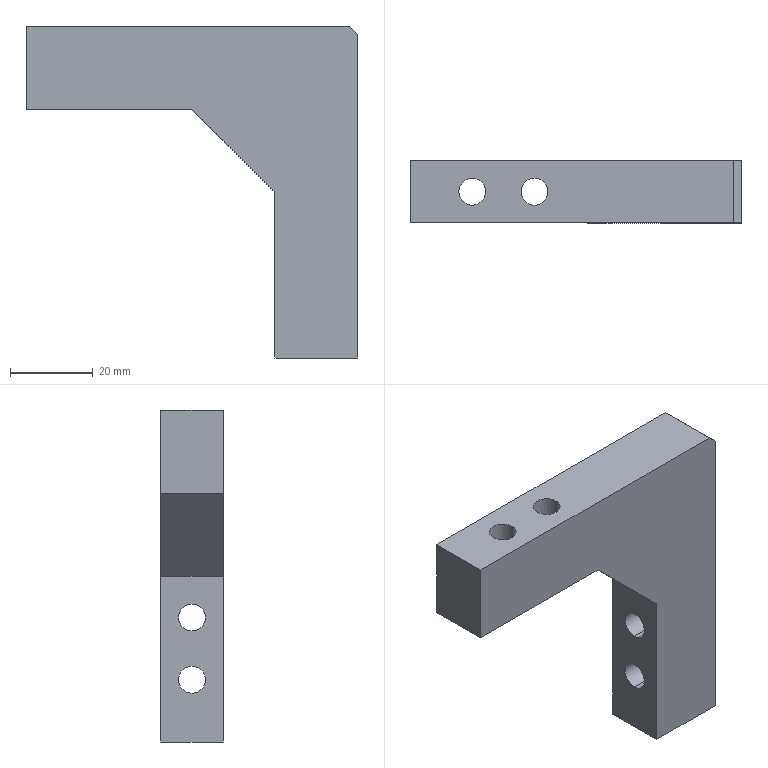Part | SolidWorks | features ICE 2, LPattern 2, Chamfer 1, Extrusion 1 | 1 solid | 18 faces | box 80 x 15 x 80 mm | volume 42315 mm3 | plane 10 | cylinder 8 | commonest cylinder face diameters 6.5 x8
STEP:
#1=CARTESIAN_POINT('',(20.,7.5,-21.75));
#2=VERTEX_POINT('',#1);
#3=CARTESIAN_POINT('',(20.,7.5,-28.25));
#4=VERTEX_POINT('',#3);
#5=CARTESIAN_POINT('',(20.,7.5,-25.));
#6=DIRECTION('',(1.,0.,0.));
#7=DIRECTION('',(0.,0.,-1.));
#8=AXIS2_PLACEMENT_3D('',#5,#6,#7);
#9=CIRCLE('',#8,3.25);
#10=EDGE_CURVE('',#2,#4,#9,.T.);
#11=ORIENTED_EDGE('',*,*,#10,.F.);
#12=CARTESIAN_POINT('',(40.,7.5,-21.75));
#13=VERTEX_POINT('',#12);
#14=CARTESIAN_POINT('',(-40.,7.5,-21.75));
#15=DIRECTION('',(1.,0.,0.));
#16=VECTOR('',#15,1000.);
#17=LINE('',#14,#16);
#18=EDGE_CURVE('',#2,#13,#17,.T.);
#19=ORIENTED_EDGE('',*,*,#18,.T.);
#20=CARTESIAN_POINT('',(40.,7.5,-28.25));
#21=VERTEX_POINT('',#20);
#22=CARTESIAN_POINT('',(40.,7.5,-25.));
#23=DIRECTION('',(1.,0.,0.));
#24=DIRECTION('',(0.,0.,-1.));
#25=AXIS2_PLACEMENT_3D('',#22,#23,#24);
#26=CIRCLE('',#25,3.25);
#27=EDGE_CURVE('',#13,#21,#26,.T.);
#28=ORIENTED_EDGE('',*,*,#27,.T.);
#29=CARTESIAN_POINT('',(-40.,7.5,-28.25));
#30=DIRECTION('',(1.,0.,0.));
#31=VECTOR('',#30,1000.);
#32=LINE('',#29,#31);
#33=EDGE_CURVE('',#4,#21,#32,.T.);
#34=ORIENTED_EDGE('',*,*,#33,.F.);
#35=EDGE_LOOP('',(#11,#19,#28,#34));
#36=FACE_OUTER_BOUND('',#35,.T.);
#37=CARTESIAN_POINT('',(-40.,7.5,-25.));
#38=DIRECTION('',(1.,0.,0.));
#39=DIRECTION('',(0.,0.,-1.));
#40=AXIS2_PLACEMENT_3D('',#37,#38,#39);
#41=CYLINDRICAL_SURFACE('',#40,3.25);
#42=ADVANCED_FACE('',(#36),#41,.F.);
#43=CARTESIAN_POINT('',(20.,7.5,-6.75));
#44=VERTEX_POINT('',#43);
#45=CARTESIAN_POINT('',(20.,7.5,-13.25));
#46=VERTEX_POINT('',#45);
#47=CARTESIAN_POINT('',(20.,7.5,-10.));
#48=DIRECTION('',(1.,0.,0.));
#49=DIRECTION('',(0.,0.,-1.));
#50=AXIS2_PLACEMENT_3D('',#47,#48,#49);
#51=CIRCLE('',#50,3.25);
#52=EDGE_CURVE('',#44,#46,#51,.T.);
#53=ORIENTED_EDGE('',*,*,#52,.F.);
#54=CARTESIAN_POINT('',(40.,7.5,-6.75));
#55=VERTEX_POINT('',#54);
#56=CARTESIAN_POINT('',(-40.,7.5,-6.75));
#57=DIRECTION('',(1.,0.,0.));
#58=VECTOR('',#57,1000.);
#59=LINE('',#56,#58);
#60=EDGE_CURVE('',#44,#55,#59,.T.);
#61=ORIENTED_EDGE('',*,*,#60,.T.);
#62=CARTESIAN_POINT('',(40.,7.5,-13.25));
#63=VERTEX_POINT('',#62);
#64=CARTESIAN_POINT('',(40.,7.5,-10.));
#65=DIRECTION('',(1.,0.,0.));
#66=DIRECTION('',(0.,0.,-1.));
#67=AXIS2_PLACEMENT_3D('',#64,#65,#66);
#68=CIRCLE('',#67,3.25);
#69=EDGE_CURVE('',#55,#63,#68,.T.);
#70=ORIENTED_EDGE('',*,*,#69,.T.);
#71=CARTESIAN_POINT('',(-40.,7.5,-13.25));
#72=DIRECTION('',(1.,0.,0.));
#73=VECTOR('',#72,1000.);
#74=LINE('',#71,#73);
#75=EDGE_CURVE('',#46,#63,#74,.T.);
#76=ORIENTED_EDGE('',*,*,#75,.F.);
#77=EDGE_LOOP('',(#53,#61,#70,#76));
#78=FACE_OUTER_BOUND('',#77,.T.);
#79=CARTESIAN_POINT('',(-40.,7.5,-10.));
#80=DIRECTION('',(1.,0.,0.));
#81=DIRECTION('',(0.,0.,-1.));
#82=AXIS2_PLACEMENT_3D('',#79,#80,#81);
#83=CYLINDRICAL_SURFACE('',#82,3.25);
#84=ADVANCED_FACE('',(#78),#83,.F.);
#85=CARTESIAN_POINT('',(-21.75,7.5,40.));
#86=VERTEX_POINT('',#85);
#87=CARTESIAN_POINT('',(-28.25,7.5,40.));
#88=VERTEX_POINT('',#87);
#89=CARTESIAN_POINT('',(-25.,7.5,40.));
#90=DIRECTION('',(0.,0.,-1.));
#91=DIRECTION('',(-1.,0.,0.));
#92=AXIS2_PLACEMENT_3D('',#89,#90,#91);
#93=CIRCLE('',#92,3.25);
#94=EDGE_CURVE('',#86,#88,#93,.T.);
#95=ORIENTED_EDGE('',*,*,#94,.F.);
#96=CARTESIAN_POINT('',(-21.75,7.5,20.));
#97=VERTEX_POINT('',#96);
#98=CARTESIAN_POINT('',(-21.75,7.5,40.));
#99=DIRECTION('',(0.,0.,-1.));
#100=VECTOR('',#99,1000.);
#101=LINE('',#98,#100);
#102=EDGE_CURVE('',#86,#97,#101,.T.);
#103=ORIENTED_EDGE('',*,*,#102,.T.);
#104=CARTESIAN_POINT('',(-28.25,7.5,20.));
#105=VERTEX_POINT('',#104);
#106=CARTESIAN_POINT('',(-25.,7.5,20.));
#107=DIRECTION('',(0.,0.,-1.));
#108=DIRECTION('',(-1.,0.,0.));
#109=AXIS2_PLACEMENT_3D('',#106,#107,#108);
#110=CIRCLE('',#109,3.25);
#111=EDGE_CURVE('',#97,#105,#110,.T.);
#112=ORIENTED_EDGE('',*,*,#111,.T.);
#113=CARTESIAN_POINT('',(-28.25,7.5,40.));
#114=DIRECTION('',(0.,0.,-1.));
#115=VECTOR('',#114,1000.);
#116=LINE('',#113,#115);
#117=EDGE_CURVE('',#88,#105,#116,.T.);
#118=ORIENTED_EDGE('',*,*,#117,.F.);
#119=EDGE_LOOP('',(#95,#103,#112,#118));
#120=FACE_OUTER_BOUND('',#119,.T.);
#121=CARTESIAN_POINT('',(-25.,7.5,40.));
#122=DIRECTION('',(0.,0.,-1.));
#123=DIRECTION('',(-1.,0.,0.));
#124=AXIS2_PLACEMENT_3D('',#121,#122,#123);
#125=CYLINDRICAL_SURFACE('',#124,3.25);
#126=ADVANCED_FACE('',(#120),#125,.F.);
#127=CARTESIAN_POINT('',(-6.75,7.5,40.));
#128=VERTEX_POINT('',#127);
#129=CARTESIAN_POINT('',(-13.25,7.5,40.));
#130=VERTEX_POINT('',#129);
#131=CARTESIAN_POINT('',(-10.,7.5,40.));
#132=DIRECTION('',(0.,0.,-1.));
#133=DIRECTION('',(-1.,0.,0.));
#134=AXIS2_PLACEMENT_3D('',#131,#132,#133);
#135=CIRCLE('',#134,3.25);
#136=EDGE_CURVE('',#128,#130,#135,.T.);
#137=ORIENTED_EDGE('',*,*,#136,.F.);
#138=CARTESIAN_POINT('',(-6.75,7.5,20.));
#139=VERTEX_POINT('',#138);
#140=CARTESIAN_POINT('',(-6.75,7.5,40.));
#141=DIRECTION('',(0.,0.,-1.));
#142=VECTOR('',#141,1000.);
#143=LINE('',#140,#142);
#144=EDGE_CURVE('',#128,#139,#143,.T.);
#145=ORIENTED_EDGE('',*,*,#144,.T.);
#146=CARTESIAN_POINT('',(-13.25,7.5,20.));
#147=VERTEX_POINT('',#146);
#148=CARTESIAN_POINT('',(-10.,7.5,20.));
#149=DIRECTION('',(0.,0.,-1.));
#150=DIRECTION('',(-1.,0.,0.));
#151=AXIS2_PLACEMENT_3D('',#148,#149,#150);
#152=CIRCLE('',#151,3.25);
#153=EDGE_CURVE('',#139,#147,#152,.T.);
#154=ORIENTED_EDGE('',*,*,#153,.T.);
#155=CARTESIAN_POINT('',(-13.25,7.5,40.));
#156=DIRECTION('',(0.,0.,-1.));
#157=VECTOR('',#156,1000.);
#158=LINE('',#155,#157);
#159=EDGE_CURVE('',#130,#147,#158,.T.);
#160=ORIENTED_EDGE('',*,*,#159,.F.);
#161=EDGE_LOOP('',(#137,#145,#154,#160));
#162=FACE_OUTER_BOUND('',#161,.T.);
#163=CARTESIAN_POINT('',(-10.,7.5,40.));
#164=DIRECTION('',(0.,0.,-1.));
#165=DIRECTION('',(-1.,0.,0.));
#166=AXIS2_PLACEMENT_3D('',#163,#164,#165);
#167=CYLINDRICAL_SURFACE('',#166,3.25);
#168=ADVANCED_FACE('',(#162),#167,.F.);
#169=CARTESIAN_POINT('',(40.,7.5,-25.));
#170=DIRECTION('',(1.,0.,0.));
#171=DIRECTION('',(0.,0.,-1.));
#172=AXIS2_PLACEMENT_3D('',#169,#170,#171);
#173=CIRCLE('',#172,3.25);
#174=EDGE_CURVE('',#21,#13,#173,.T.);
#175=ORIENTED_EDGE('',*,*,#174,.F.);
#176=ORIENTED_EDGE('',*,*,#27,.F.);
#177=EDGE_LOOP('',(#175,#176));
#178=FACE_BOUND('',#177,.T.);
#179=CARTESIAN_POINT('',(40.,7.5,-10.));
#180=DIRECTION('',(1.,0.,0.));
#181=DIRECTION('',(0.,0.,-1.));
#182=AXIS2_PLACEMENT_3D('',#179,#180,#181);
#183=CIRCLE('',#182,3.25);
#184=EDGE_CURVE('',#63,#55,#183,.T.);
#185=ORIENTED_EDGE('',*,*,#184,.F.);
#186=ORIENTED_EDGE('',*,*,#69,.F.);
#187=EDGE_LOOP('',(#185,#186));
#188=FACE_BOUND('',#187,.T.);
#189=CARTESIAN_POINT('',(40.,15.,38.));
#190=VERTEX_POINT('',#189);
#191=CARTESIAN_POINT('',(40.,15.,-40.));
#192=VERTEX_POINT('',#191);
#193=CARTESIAN_POINT('',(40.,15.,40.));
#194=DIRECTION('',(0.,0.,-1.));
#195=VECTOR('',#194,1000.);
#196=LINE('',#193,#195);
#197=EDGE_CURVE('',#190,#192,#196,.T.);
#198=ORIENTED_EDGE('',*,*,#197,.F.);
#199=CARTESIAN_POINT('',(40.,0.,38.));
#200=VERTEX_POINT('',#199);
#201=CARTESIAN_POINT('',(40.,15.,38.));
#202=DIRECTION('',(0.,-1.,0.));
#203=VECTOR('',#202,1000.);
#204=LINE('',#201,#203);
#205=EDGE_CURVE('',#190,#200,#204,.T.);
#206=ORIENTED_EDGE('',*,*,#205,.T.);
#207=CARTESIAN_POINT('',(40.,0.,-40.));
#208=VERTEX_POINT('',#207);
#209=CARTESIAN_POINT('',(40.,0.,40.));
#210=DIRECTION('',(0.,0.,-1.));
#211=VECTOR('',#210,1000.);
#212=LINE('',#209,#211);
#213=EDGE_CURVE('',#200,#208,#212,.T.);
#214=ORIENTED_EDGE('',*,*,#213,.T.);
#215=CARTESIAN_POINT('',(40.,15.,-40.));
#216=DIRECTION('',(0.,-1.,0.));
#217=VECTOR('',#216,1000.);
#218=LINE('',#215,#217);
#219=EDGE_CURVE('',#192,#208,#218,.T.);
#220=ORIENTED_EDGE('',*,*,#219,.F.);
#221=EDGE_LOOP('',(#198,#206,#214,#220));
#222=FACE_OUTER_BOUND('',#221,.T.);
#223=CARTESIAN_POINT('',(40.,15.,40.));
#224=DIRECTION('',(-1.,0.,0.));
#225=DIRECTION('',(0.,0.,1.));
#226=AXIS2_PLACEMENT_3D('',#223,#224,#225);
#227=PLANE('',#226);
#228=ADVANCED_FACE('',(#178,#188,#222),#227,.F.);
#229=CARTESIAN_POINT('',(20.,0.,-40.));
#230=VERTEX_POINT('',#229);
#231=CARTESIAN_POINT('',(40.,0.,-40.));
#232=DIRECTION('',(-1.,0.,0.));
#233=VECTOR('',#232,1000.);
#234=LINE('',#231,#233);
#235=EDGE_CURVE('',#208,#230,#234,.T.);
#236=ORIENTED_EDGE('',*,*,#235,.T.);
#237=CARTESIAN_POINT('',(20.,15.,-40.));
#238=VERTEX_POINT('',#237);
#239=CARTESIAN_POINT('',(20.,15.,-40.));
#240=DIRECTION('',(0.,-1.,0.));
#241=VECTOR('',#240,1000.);
#242=LINE('',#239,#241);
#243=EDGE_CURVE('',#238,#230,#242,.T.);
#244=ORIENTED_EDGE('',*,*,#243,.F.);
#245=CARTESIAN_POINT('',(40.,15.,-40.));
#246=DIRECTION('',(-1.,0.,0.));
#247=VECTOR('',#246,1000.);
#248=LINE('',#245,#247);
#249=EDGE_CURVE('',#192,#238,#248,.T.);
#250=ORIENTED_EDGE('',*,*,#249,.F.);
#251=ORIENTED_EDGE('',*,*,#219,.T.);
#252=EDGE_LOOP('',(#236,#244,#250,#251));
#253=FACE_OUTER_BOUND('',#252,.T.);
#254=CARTESIAN_POINT('',(40.,15.,-40.));
#255=DIRECTION('',(0.,0.,1.));
#256=DIRECTION('',(1.,0.,0.));
#257=AXIS2_PLACEMENT_3D('',#254,#255,#256);
#258=PLANE('',#257);
#259=ADVANCED_FACE('',(#253),#258,.F.);
#260=CARTESIAN_POINT('',(20.,7.5,-25.));
#261=DIRECTION('',(1.,0.,0.));
#262=DIRECTION('',(0.,0.,-1.));
#263=AXIS2_PLACEMENT_3D('',#260,#261,#262);
#264=CIRCLE('',#263,3.25);
#265=EDGE_CURVE('',#4,#2,#264,.T.);
#266=ORIENTED_EDGE('',*,*,#265,.T.);
#267=ORIENTED_EDGE('',*,*,#10,.T.);
#268=EDGE_LOOP('',(#266,#267));
#269=FACE_BOUND('',#268,.T.);
#270=CARTESIAN_POINT('',(20.,7.5,-10.));
#271=DIRECTION('',(1.,0.,0.));
#272=DIRECTION('',(0.,0.,-1.));
#273=AXIS2_PLACEMENT_3D('',#270,#271,#272);
#274=CIRCLE('',#273,3.25);
#275=EDGE_CURVE('',#46,#44,#274,.T.);
#276=ORIENTED_EDGE('',*,*,#275,.T.);
#277=ORIENTED_EDGE('',*,*,#52,.T.);
#278=EDGE_LOOP('',(#276,#277));
#279=FACE_BOUND('',#278,.T.);
#280=CARTESIAN_POINT('',(20.,0.,0.));
#281=VERTEX_POINT('',#280);
#282=CARTESIAN_POINT('',(20.,0.,-40.));
#283=DIRECTION('',(0.,0.,1.));
#284=VECTOR('',#283,1000.);
#285=LINE('',#282,#284);
#286=EDGE_CURVE('',#230,#281,#285,.T.);
#287=ORIENTED_EDGE('',*,*,#286,.T.);
#288=CARTESIAN_POINT('',(20.,15.,0.));
#289=VERTEX_POINT('',#288);
#290=CARTESIAN_POINT('',(20.,15.,0.));
#291=DIRECTION('',(0.,-1.,0.));
#292=VECTOR('',#291,1000.);
#293=LINE('',#290,#292);
#294=EDGE_CURVE('',#289,#281,#293,.T.);
#295=ORIENTED_EDGE('',*,*,#294,.F.);
#296=CARTESIAN_POINT('',(20.,15.,-40.));
#297=DIRECTION('',(0.,0.,1.));
#298=VECTOR('',#297,1000.);
#299=LINE('',#296,#298);
#300=EDGE_CURVE('',#238,#289,#299,.T.);
#301=ORIENTED_EDGE('',*,*,#300,.F.);
#302=ORIENTED_EDGE('',*,*,#243,.T.);
#303=EDGE_LOOP('',(#287,#295,#301,#302));
#304=FACE_OUTER_BOUND('',#303,.T.);
#305=CARTESIAN_POINT('',(20.,15.,-40.));
#306=DIRECTION('',(1.,0.,0.));
#307=DIRECTION('',(0.,0.,-1.));
#308=AXIS2_PLACEMENT_3D('',#305,#306,#307);
#309=PLANE('',#308);
#310=ADVANCED_FACE('',(#269,#279,#304),#309,.F.);
#311=CARTESIAN_POINT('',(0.,0.,20.));
#312=VERTEX_POINT('',#311);
#313=CARTESIAN_POINT('',(20.,0.,0.));
#314=DIRECTION('',(-0.7071,0.,0.7071));
#315=VECTOR('',#314,1000.);
#316=LINE('',#313,#315);
#317=EDGE_CURVE('',#281,#312,#316,.T.);
#318=ORIENTED_EDGE('',*,*,#317,.T.);
#319=CARTESIAN_POINT('',(0.,15.,20.));
#320=VERTEX_POINT('',#319);
#321=CARTESIAN_POINT('',(0.,15.,20.));
#322=DIRECTION('',(0.,-1.,0.));
#323=VECTOR('',#322,1000.);
#324=LINE('',#321,#323);
#325=EDGE_CURVE('',#320,#312,#324,.T.);
#326=ORIENTED_EDGE('',*,*,#325,.F.);
#327=CARTESIAN_POINT('',(20.,15.,0.));
#328=DIRECTION('',(-0.7071,0.,0.7071));
#329=VECTOR('',#328,1000.);
#330=LINE('',#327,#329);
#331=EDGE_CURVE('',#289,#320,#330,.T.);
#332=ORIENTED_EDGE('',*,*,#331,.F.);
#333=ORIENTED_EDGE('',*,*,#294,.T.);
#334=EDGE_LOOP('',(#318,#326,#332,#333));
#335=FACE_OUTER_BOUND('',#334,.T.);
#336=CARTESIAN_POINT('',(20.,15.,0.));
#337=DIRECTION('',(0.7071,0.,0.7071));
#338=DIRECTION('',(0.7071,0.,-0.7071));
#339=AXIS2_PLACEMENT_3D('',#336,#337,#338);
#340=PLANE('',#339);
#341=ADVANCED_FACE('',(#335),#340,.F.);
#342=CARTESIAN_POINT('',(-25.,7.5,20.));
#343=DIRECTION('',(0.,0.,-1.));
#344=DIRECTION('',(-1.,0.,0.));
#345=AXIS2_PLACEMENT_3D('',#342,#343,#344);
#346=CIRCLE('',#345,3.25);
#347=EDGE_CURVE('',#105,#97,#346,.T.);
#348=ORIENTED_EDGE('',*,*,#347,.F.);
#349=ORIENTED_EDGE('',*,*,#111,.F.);
#350=EDGE_LOOP('',(#348,#349));
#351=FACE_BOUND('',#350,.T.);
#352=CARTESIAN_POINT('',(-10.,7.5,20.));
#353=DIRECTION('',(0.,0.,-1.));
#354=DIRECTION('',(-1.,0.,0.));
#355=AXIS2_PLACEMENT_3D('',#352,#353,#354);
#356=CIRCLE('',#355,3.25);
#357=EDGE_CURVE('',#147,#139,#356,.T.);
#358=ORIENTED_EDGE('',*,*,#357,.F.);
#359=ORIENTED_EDGE('',*,*,#153,.F.);
#360=EDGE_LOOP('',(#358,#359));
#361=FACE_BOUND('',#360,.T.);
#362=CARTESIAN_POINT('',(-40.,0.,20.));
#363=VERTEX_POINT('',#362);
#364=CARTESIAN_POINT('',(0.,0.,20.));
#365=DIRECTION('',(-1.,0.,0.));
#366=VECTOR('',#365,1000.);
#367=LINE('',#364,#366);
#368=EDGE_CURVE('',#312,#363,#367,.T.);
#369=ORIENTED_EDGE('',*,*,#368,.T.);
#370=CARTESIAN_POINT('',(-40.,15.,20.));
#371=VERTEX_POINT('',#370);
#372=CARTESIAN_POINT('',(-40.,15.,20.));
#373=DIRECTION('',(0.,-1.,0.));
#374=VECTOR('',#373,1000.);
#375=LINE('',#372,#374);
#376=EDGE_CURVE('',#371,#363,#375,.T.);
#377=ORIENTED_EDGE('',*,*,#376,.F.);
#378=CARTESIAN_POINT('',(0.,15.,20.));
#379=DIRECTION('',(-1.,0.,0.));
#380=VECTOR('',#379,1000.);
#381=LINE('',#378,#380);
#382=EDGE_CURVE('',#320,#371,#381,.T.);
#383=ORIENTED_EDGE('',*,*,#382,.F.);
#384=ORIENTED_EDGE('',*,*,#325,.T.);
#385=EDGE_LOOP('',(#369,#377,#383,#384));
#386=FACE_OUTER_BOUND('',#385,.T.);
#387=CARTESIAN_POINT('',(0.,15.,20.));
#388=DIRECTION('',(0.,0.,1.));
#389=DIRECTION('',(1.,0.,0.));
#390=AXIS2_PLACEMENT_3D('',#387,#388,#389);
#391=PLANE('',#390);
#392=ADVANCED_FACE('',(#351,#361,#386),#391,.F.);
#393=CARTESIAN_POINT('',(-40.,0.,40.));
#394=VERTEX_POINT('',#393);
#395=CARTESIAN_POINT('',(-40.,0.,40.));
#396=DIRECTION('',(0.,0.,1.));
#397=VECTOR('',#396,1000.);
#398=LINE('',#395,#397);
#399=EDGE_CURVE('',#363,#394,#398,.T.);
#400=ORIENTED_EDGE('',*,*,#399,.T.);
#401=CARTESIAN_POINT('',(-40.,15.,40.));
#402=VERTEX_POINT('',#401);
#403=CARTESIAN_POINT('',(-40.,15.,40.));
#404=DIRECTION('',(0.,-1.,0.));
#405=VECTOR('',#404,1000.);
#406=LINE('',#403,#405);
#407=EDGE_CURVE('',#402,#394,#406,.T.);
#408=ORIENTED_EDGE('',*,*,#407,.F.);
#409=CARTESIAN_POINT('',(-40.,15.,40.));
#410=DIRECTION('',(0.,0.,1.));
#411=VECTOR('',#410,1000.);
#412=LINE('',#409,#411);
#413=EDGE_CURVE('',#371,#402,#412,.T.);
#414=ORIENTED_EDGE('',*,*,#413,.F.);
#415=ORIENTED_EDGE('',*,*,#376,.T.);
#416=EDGE_LOOP('',(#400,#408,#414,#415));
#417=FACE_OUTER_BOUND('',#416,.T.);
#418=CARTESIAN_POINT('',(-40.,15.,40.));
#419=DIRECTION('',(1.,0.,0.));
#420=DIRECTION('',(0.,0.,-1.));
#421=AXIS2_PLACEMENT_3D('',#418,#419,#420);
#422=PLANE('',#421);
#423=ADVANCED_FACE('',(#417),#422,.F.);
#424=CARTESIAN_POINT('',(-25.,7.5,40.));
#425=DIRECTION('',(0.,0.,-1.));
#426=DIRECTION('',(-1.,0.,0.));
#427=AXIS2_PLACEMENT_3D('',#424,#425,#426);
#428=CIRCLE('',#427,3.25);
#429=EDGE_CURVE('',#88,#86,#428,.T.);
#430=ORIENTED_EDGE('',*,*,#429,.T.);
#431=ORIENTED_EDGE('',*,*,#94,.T.);
#432=EDGE_LOOP('',(#430,#431));
#433=FACE_BOUND('',#432,.T.);
#434=CARTESIAN_POINT('',(-10.,7.5,40.));
#435=DIRECTION('',(0.,0.,-1.));
#436=DIRECTION('',(-1.,0.,0.));
#437=AXIS2_PLACEMENT_3D('',#434,#435,#436);
#438=CIRCLE('',#437,3.25);
#439=EDGE_CURVE('',#130,#128,#438,.T.);
#440=ORIENTED_EDGE('',*,*,#439,.T.);
#441=ORIENTED_EDGE('',*,*,#136,.T.);
#442=EDGE_LOOP('',(#440,#441));
#443=FACE_BOUND('',#442,.T.);
#444=CARTESIAN_POINT('',(38.,0.,40.));
#445=VERTEX_POINT('',#444);
#446=CARTESIAN_POINT('',(-40.,0.,40.));
#447=DIRECTION('',(1.,0.,0.));
#448=VECTOR('',#447,1000.);
#449=LINE('',#446,#448);
#450=EDGE_CURVE('',#394,#445,#449,.T.);
#451=ORIENTED_EDGE('',*,*,#450,.T.);
#452=CARTESIAN_POINT('',(38.,15.,40.));
#453=VERTEX_POINT('',#452);
#454=CARTESIAN_POINT('',(38.,15.,40.));
#455=DIRECTION('',(0.,1.,0.));
#456=VECTOR('',#455,1000.);
#457=LINE('',#454,#456);
#458=EDGE_CURVE('',#445,#453,#457,.T.);
#459=ORIENTED_EDGE('',*,*,#458,.T.);
#460=CARTESIAN_POINT('',(-40.,15.,40.));
#461=DIRECTION('',(1.,0.,0.));
#462=VECTOR('',#461,1000.);
#463=LINE('',#460,#462);
#464=EDGE_CURVE('',#402,#453,#463,.T.);
#465=ORIENTED_EDGE('',*,*,#464,.F.);
#466=ORIENTED_EDGE('',*,*,#407,.T.);
#467=EDGE_LOOP('',(#451,#459,#465,#466));
#468=FACE_OUTER_BOUND('',#467,.T.);
#469=CARTESIAN_POINT('',(-40.,15.,40.));
#470=DIRECTION('',(0.,0.,-1.));
#471=DIRECTION('',(-1.,0.,0.));
#472=AXIS2_PLACEMENT_3D('',#469,#470,#471);
#473=PLANE('',#472);
#474=ADVANCED_FACE('',(#433,#443,#468),#473,.F.);
#475=ORIENTED_EDGE('',*,*,#464,.T.);
#476=CARTESIAN_POINT('',(79.,15.,-1.));
#477=DIRECTION('',(0.7071,0.,-0.7071));
#478=VECTOR('',#477,1000.);
#479=LINE('',#476,#478);
#480=EDGE_CURVE('',#453,#190,#479,.T.);
#481=ORIENTED_EDGE('',*,*,#480,.T.);
#482=ORIENTED_EDGE('',*,*,#197,.T.);
#483=ORIENTED_EDGE('',*,*,#249,.T.);
#484=ORIENTED_EDGE('',*,*,#300,.T.);
#485=ORIENTED_EDGE('',*,*,#331,.T.);
#486=ORIENTED_EDGE('',*,*,#382,.T.);
#487=ORIENTED_EDGE('',*,*,#413,.T.);
#488=EDGE_LOOP('',(#475,#481,#482,#483,#484,#485,#486,#487));
#489=FACE_OUTER_BOUND('',#488,.T.);
#490=CARTESIAN_POINT('',(40.,15.,-40.));
#491=DIRECTION('',(0.,1.,0.));
#492=DIRECTION('',(0.,0.,1.));
#493=AXIS2_PLACEMENT_3D('',#490,#491,#492);
#494=PLANE('',#493);
#495=ADVANCED_FACE('',(#489),#494,.T.);
#496=ORIENTED_EDGE('',*,*,#213,.F.);
#497=CARTESIAN_POINT('',(40.,0.,38.));
#498=DIRECTION('',(-0.7071,0.,0.7071));
#499=VECTOR('',#498,1000.);
#500=LINE('',#497,#499);
#501=EDGE_CURVE('',#200,#445,#500,.T.);
#502=ORIENTED_EDGE('',*,*,#501,.T.);
#503=ORIENTED_EDGE('',*,*,#450,.F.);
#504=ORIENTED_EDGE('',*,*,#399,.F.);
#505=ORIENTED_EDGE('',*,*,#368,.F.);
#506=ORIENTED_EDGE('',*,*,#317,.F.);
#507=ORIENTED_EDGE('',*,*,#286,.F.);
#508=ORIENTED_EDGE('',*,*,#235,.F.);
#509=EDGE_LOOP('',(#496,#502,#503,#504,#505,#506,#507,#508));
#510=FACE_OUTER_BOUND('',#509,.T.);
#511=CARTESIAN_POINT('',(40.,0.,-40.));
#512=DIRECTION('',(0.,1.,0.));
#513=DIRECTION('',(0.,0.,1.));
#514=AXIS2_PLACEMENT_3D('',#511,#512,#513);
#515=PLANE('',#514);
#516=ADVANCED_FACE('',(#510),#515,.F.);
#517=ORIENTED_EDGE('',*,*,#144,.F.);
#518=ORIENTED_EDGE('',*,*,#439,.F.);
#519=ORIENTED_EDGE('',*,*,#159,.T.);
#520=ORIENTED_EDGE('',*,*,#357,.T.);
#521=EDGE_LOOP('',(#517,#518,#519,#520));
#522=FACE_OUTER_BOUND('',#521,.T.);
#523=CARTESIAN_POINT('',(-10.,7.5,40.));
#524=DIRECTION('',(0.,0.,-1.));
#525=DIRECTION('',(-1.,0.,0.));
#526=AXIS2_PLACEMENT_3D('',#523,#524,#525);
#527=CYLINDRICAL_SURFACE('',#526,3.25);
#528=ADVANCED_FACE('',(#522),#527,.F.);
#529=ORIENTED_EDGE('',*,*,#102,.F.);
#530=ORIENTED_EDGE('',*,*,#429,.F.);
#531=ORIENTED_EDGE('',*,*,#117,.T.);
#532=ORIENTED_EDGE('',*,*,#347,.T.);
#533=EDGE_LOOP('',(#529,#530,#531,#532));
#534=FACE_OUTER_BOUND('',#533,.T.);
#535=CARTESIAN_POINT('',(-25.,7.5,40.));
#536=DIRECTION('',(0.,0.,-1.));
#537=DIRECTION('',(-1.,0.,0.));
#538=AXIS2_PLACEMENT_3D('',#535,#536,#537);
#539=CYLINDRICAL_SURFACE('',#538,3.25);
#540=ADVANCED_FACE('',(#534),#539,.F.);
#541=ORIENTED_EDGE('',*,*,#60,.F.);
#542=ORIENTED_EDGE('',*,*,#275,.F.);
#543=ORIENTED_EDGE('',*,*,#75,.T.);
#544=ORIENTED_EDGE('',*,*,#184,.T.);
#545=EDGE_LOOP('',(#541,#542,#543,#544));
#546=FACE_OUTER_BOUND('',#545,.T.);
#547=CARTESIAN_POINT('',(-40.,7.5,-10.));
#548=DIRECTION('',(1.,0.,0.));
#549=DIRECTION('',(0.,0.,-1.));
#550=AXIS2_PLACEMENT_3D('',#547,#548,#549);
#551=CYLINDRICAL_SURFACE('',#550,3.25);
#552=ADVANCED_FACE('',(#546),#551,.F.);
#553=ORIENTED_EDGE('',*,*,#18,.F.);
#554=ORIENTED_EDGE('',*,*,#265,.F.);
#555=ORIENTED_EDGE('',*,*,#33,.T.);
#556=ORIENTED_EDGE('',*,*,#174,.T.);
#557=EDGE_LOOP('',(#553,#554,#555,#556));
#558=FACE_OUTER_BOUND('',#557,.T.);
#559=CARTESIAN_POINT('',(-40.,7.5,-25.));
#560=DIRECTION('',(1.,0.,0.));
#561=DIRECTION('',(0.,0.,-1.));
#562=AXIS2_PLACEMENT_3D('',#559,#560,#561);
#563=CYLINDRICAL_SURFACE('',#562,3.25);
#564=ADVANCED_FACE('',(#558),#563,.F.);
#565=ORIENTED_EDGE('',*,*,#480,.F.);
#566=ORIENTED_EDGE('',*,*,#458,.F.);
#567=ORIENTED_EDGE('',*,*,#501,.F.);
#568=ORIENTED_EDGE('',*,*,#205,.F.);
#569=EDGE_LOOP('',(#565,#566,#567,#568));
#570=FACE_OUTER_BOUND('',#569,.T.);
#571=CARTESIAN_POINT('',(40.,15.,38.));
#572=DIRECTION('',(-0.7071,0.,-0.7071));
#573=DIRECTION('',(-0.7071,0.,0.7071));
#574=AXIS2_PLACEMENT_3D('',#571,#572,#573);
#575=PLANE('',#574);
#576=ADVANCED_FACE('',(#570),#575,.F.);
#577=CLOSED_SHELL('',(#42,#84,#126,#168,#228,#259,#310,#341,#392,#423,#474,#495,#516,#528,#540,#552,#564,#576));
#578=MANIFOLD_SOLID_BREP('',#577);
#579=CARTESIAN_POINT('',(0.,0.,0.));
#580=DIRECTION('',(0.,0.,1.));
#581=DIRECTION('',(1.,0.,0.));
#582=AXIS2_PLACEMENT_3D('',#579,#580,#581);
#583=(LENGTH_UNIT()NAMED_UNIT(*)SI_UNIT(.MILLI.,.METRE.));
#584=UNCERTAINTY_MEASURE_WITH_UNIT(LENGTH_MEASURE(0.00001),#583,'','');
#585=(NAMED_UNIT(*)PLANE_ANGLE_UNIT()SI_UNIT($,.RADIAN.));
#586=(NAMED_UNIT(*)SI_UNIT($,.STERADIAN.)SOLID_ANGLE_UNIT());
#587=(GEOMETRIC_REPRESENTATION_CONTEXT(3)GLOBAL_UNCERTAINTY_ASSIGNED_CONTEXT((#584))GLOBAL_UNIT_ASSIGNED_CONTEXT((#583,#585,#586))REPRESENTATION_CONTEXT('',''));
#588=ADVANCED_BREP_SHAPE_REPRESENTATION('',(#578,#582),#587);